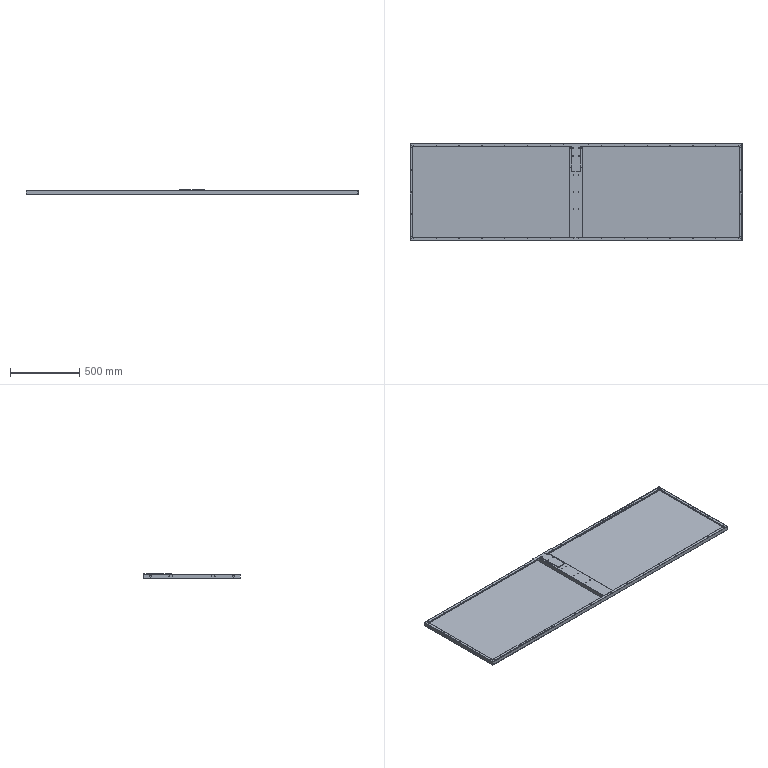Part | NX | features BREP 4 | 4 solids | 252 faces | box 2400 x 700 x 36 mm | volume 2270494 mm3 | cylinder 172 | plane 64 | spline 16 | commonest cylinder face diameters 3.3 x104 6.8 x20 6.6 x16 1.473 x8 3.473 x8 11 x8